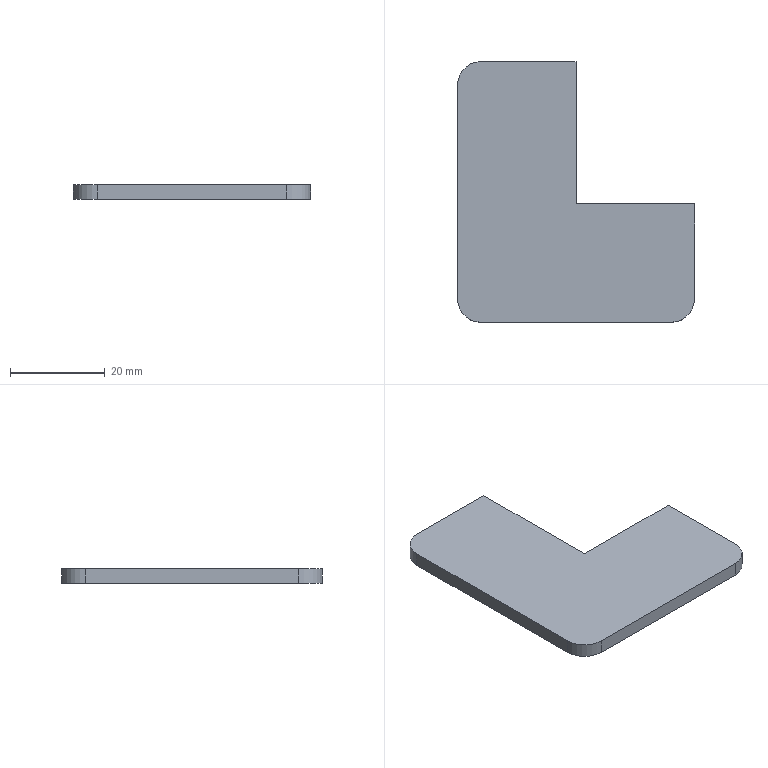Part | SolidWorks | features Extrusion 1 | 1 solid | 11 faces | box 50 x 55 x 3 mm | volume 5952 mm3 | plane 8 | cylinder 3 | commonest cylinder face diameters 10 x3
STEP:
#1=CARTESIAN_POINT('',(-360.,-23.,0.));
#2=VERTEX_POINT('',#1);
#3=CARTESIAN_POINT('',(-360.,-3.,0.));
#4=VERTEX_POINT('',#3);
#5=CARTESIAN_POINT('',(-360.,-3.,0.));
#6=DIRECTION('',(0.,1.,0.));
#7=VECTOR('',#6,1000.);
#8=LINE('',#5,#7);
#9=EDGE_CURVE('',#2,#4,#8,.T.);
#10=ORIENTED_EDGE('',*,*,#9,.T.);
#11=CARTESIAN_POINT('',(-360.,-3.,3.));
#12=VERTEX_POINT('',#11);
#13=CARTESIAN_POINT('',(-360.,-3.,3.));
#14=DIRECTION('',(0.,0.,-1.));
#15=VECTOR('',#14,1000.);
#16=LINE('',#13,#15);
#17=EDGE_CURVE('',#12,#4,#16,.T.);
#18=ORIENTED_EDGE('',*,*,#17,.F.);
#19=CARTESIAN_POINT('',(-360.,-23.,3.));
#20=VERTEX_POINT('',#19);
#21=CARTESIAN_POINT('',(-360.,-3.,3.));
#22=DIRECTION('',(0.,1.,0.));
#23=VECTOR('',#22,1000.);
#24=LINE('',#21,#23);
#25=EDGE_CURVE('',#20,#12,#24,.T.);
#26=ORIENTED_EDGE('',*,*,#25,.F.);
#27=CARTESIAN_POINT('',(-360.,-23.,3.));
#28=DIRECTION('',(0.,0.,-1.));
#29=VECTOR('',#28,1000.);
#30=LINE('',#27,#29);
#31=EDGE_CURVE('',#20,#2,#30,.T.);
#32=ORIENTED_EDGE('',*,*,#31,.T.);
#33=EDGE_LOOP('',(#10,#18,#26,#32));
#34=FACE_OUTER_BOUND('',#33,.T.);
#35=CARTESIAN_POINT('',(-360.,-3.,3.));
#36=DIRECTION('',(-1.,0.,0.));
#37=DIRECTION('',(0.,0.,1.));
#38=AXIS2_PLACEMENT_3D('',#35,#36,#37);
#39=PLANE('',#38);
#40=ADVANCED_FACE('',(#34),#39,.F.);
#41=CARTESIAN_POINT('',(-385.,-3.,0.));
#42=VERTEX_POINT('',#41);
#43=CARTESIAN_POINT('',(-360.,-3.,0.));
#44=DIRECTION('',(-1.,0.,0.));
#45=VECTOR('',#44,1000.);
#46=LINE('',#43,#45);
#47=EDGE_CURVE('',#4,#42,#46,.T.);
#48=ORIENTED_EDGE('',*,*,#47,.T.);
#49=CARTESIAN_POINT('',(-385.,-3.,3.));
#50=VERTEX_POINT('',#49);
#51=CARTESIAN_POINT('',(-385.,-3.,3.));
#52=DIRECTION('',(0.,0.,-1.));
#53=VECTOR('',#52,1000.);
#54=LINE('',#51,#53);
#55=EDGE_CURVE('',#50,#42,#54,.T.);
#56=ORIENTED_EDGE('',*,*,#55,.F.);
#57=CARTESIAN_POINT('',(-360.,-3.,3.));
#58=DIRECTION('',(-1.,0.,0.));
#59=VECTOR('',#58,1000.);
#60=LINE('',#57,#59);
#61=EDGE_CURVE('',#12,#50,#60,.T.);
#62=ORIENTED_EDGE('',*,*,#61,.F.);
#63=ORIENTED_EDGE('',*,*,#17,.T.);
#64=EDGE_LOOP('',(#48,#56,#62,#63));
#65=FACE_OUTER_BOUND('',#64,.T.);
#66=CARTESIAN_POINT('',(-360.,-3.,3.));
#67=DIRECTION('',(0.,-1.,0.));
#68=DIRECTION('',(1.,0.,0.));
#69=AXIS2_PLACEMENT_3D('',#66,#67,#68);
#70=PLANE('',#69);
#71=ADVANCED_FACE('',(#65),#70,.F.);
#72=CARTESIAN_POINT('',(-385.,27.,0.));
#73=VERTEX_POINT('',#72);
#74=CARTESIAN_POINT('',(-385.,27.,0.));
#75=DIRECTION('',(0.,1.,0.));
#76=VECTOR('',#75,1000.);
#77=LINE('',#74,#76);
#78=EDGE_CURVE('',#42,#73,#77,.T.);
#79=ORIENTED_EDGE('',*,*,#78,.T.);
#80=CARTESIAN_POINT('',(-385.,27.,3.));
#81=VERTEX_POINT('',#80);
#82=CARTESIAN_POINT('',(-385.,27.,3.));
#83=DIRECTION('',(0.,0.,-1.));
#84=VECTOR('',#83,1000.);
#85=LINE('',#82,#84);
#86=EDGE_CURVE('',#81,#73,#85,.T.);
#87=ORIENTED_EDGE('',*,*,#86,.F.);
#88=CARTESIAN_POINT('',(-385.,27.,3.));
#89=DIRECTION('',(0.,1.,0.));
#90=VECTOR('',#89,1000.);
#91=LINE('',#88,#90);
#92=EDGE_CURVE('',#50,#81,#91,.T.);
#93=ORIENTED_EDGE('',*,*,#92,.F.);
#94=ORIENTED_EDGE('',*,*,#55,.T.);
#95=EDGE_LOOP('',(#79,#87,#93,#94));
#96=FACE_OUTER_BOUND('',#95,.T.);
#97=CARTESIAN_POINT('',(-385.,27.,3.));
#98=DIRECTION('',(-1.,0.,0.));
#99=DIRECTION('',(0.,0.,1.));
#100=AXIS2_PLACEMENT_3D('',#97,#98,#99);
#101=PLANE('',#100);
#102=ADVANCED_FACE('',(#96),#101,.F.);
#103=CARTESIAN_POINT('',(-405.,27.,0.));
#104=VERTEX_POINT('',#103);
#105=CARTESIAN_POINT('',(-385.,27.,0.));
#106=DIRECTION('',(-1.,0.,0.));
#107=VECTOR('',#106,1000.);
#108=LINE('',#105,#107);
#109=EDGE_CURVE('',#73,#104,#108,.T.);
#110=ORIENTED_EDGE('',*,*,#109,.T.);
#111=CARTESIAN_POINT('',(-405.,27.,3.));
#112=VERTEX_POINT('',#111);
#113=CARTESIAN_POINT('',(-405.,27.,3.));
#114=DIRECTION('',(0.,0.,-1.));
#115=VECTOR('',#114,1000.);
#116=LINE('',#113,#115);
#117=EDGE_CURVE('',#112,#104,#116,.T.);
#118=ORIENTED_EDGE('',*,*,#117,.F.);
#119=CARTESIAN_POINT('',(-385.,27.,3.));
#120=DIRECTION('',(-1.,0.,0.));
#121=VECTOR('',#120,1000.);
#122=LINE('',#119,#121);
#123=EDGE_CURVE('',#81,#112,#122,.T.);
#124=ORIENTED_EDGE('',*,*,#123,.F.);
#125=ORIENTED_EDGE('',*,*,#86,.T.);
#126=EDGE_LOOP('',(#110,#118,#124,#125));
#127=FACE_OUTER_BOUND('',#126,.T.);
#128=CARTESIAN_POINT('',(-385.,27.,3.));
#129=DIRECTION('',(0.,-1.,0.));
#130=DIRECTION('',(1.,0.,0.));
#131=AXIS2_PLACEMENT_3D('',#128,#129,#130);
#132=PLANE('',#131);
#133=ADVANCED_FACE('',(#127),#132,.F.);
#134=CARTESIAN_POINT('',(-410.,22.,0.));
#135=VERTEX_POINT('',#134);
#136=CARTESIAN_POINT('',(-405.,22.,0.));
#137=DIRECTION('',(0.,0.,1.));
#138=DIRECTION('',(1.,0.,0.));
#139=AXIS2_PLACEMENT_3D('',#136,#137,#138);
#140=CIRCLE('',#139,5.);
#141=EDGE_CURVE('',#104,#135,#140,.T.);
#142=ORIENTED_EDGE('',*,*,#141,.T.);
#143=CARTESIAN_POINT('',(-410.,22.,3.));
#144=VERTEX_POINT('',#143);
#145=CARTESIAN_POINT('',(-410.,22.,3.));
#146=DIRECTION('',(0.,0.,-1.));
#147=VECTOR('',#146,1000.);
#148=LINE('',#145,#147);
#149=EDGE_CURVE('',#144,#135,#148,.T.);
#150=ORIENTED_EDGE('',*,*,#149,.F.);
#151=CARTESIAN_POINT('',(-405.,22.,3.));
#152=DIRECTION('',(0.,0.,1.));
#153=DIRECTION('',(1.,0.,0.));
#154=AXIS2_PLACEMENT_3D('',#151,#152,#153);
#155=CIRCLE('',#154,5.);
#156=EDGE_CURVE('',#112,#144,#155,.T.);
#157=ORIENTED_EDGE('',*,*,#156,.F.);
#158=ORIENTED_EDGE('',*,*,#117,.T.);
#159=EDGE_LOOP('',(#142,#150,#157,#158));
#160=FACE_OUTER_BOUND('',#159,.T.);
#161=CARTESIAN_POINT('',(-405.,22.,3.));
#162=DIRECTION('',(0.,0.,-1.));
#163=DIRECTION('',(-1.,0.,0.));
#164=AXIS2_PLACEMENT_3D('',#161,#162,#163);
#165=CYLINDRICAL_SURFACE('',#164,5.);
#166=ADVANCED_FACE('',(#160),#165,.T.);
#167=CARTESIAN_POINT('',(-410.,-23.,0.));
#168=VERTEX_POINT('',#167);
#169=CARTESIAN_POINT('',(-410.,-3.,0.));
#170=DIRECTION('',(0.,-1.,0.));
#171=VECTOR('',#170,1000.);
#172=LINE('',#169,#171);
#173=EDGE_CURVE('',#135,#168,#172,.T.);
#174=ORIENTED_EDGE('',*,*,#173,.T.);
#175=CARTESIAN_POINT('',(-410.,-23.,3.));
#176=VERTEX_POINT('',#175);
#177=CARTESIAN_POINT('',(-410.,-23.,3.));
#178=DIRECTION('',(0.,0.,-1.));
#179=VECTOR('',#178,1000.);
#180=LINE('',#177,#179);
#181=EDGE_CURVE('',#176,#168,#180,.T.);
#182=ORIENTED_EDGE('',*,*,#181,.F.);
#183=CARTESIAN_POINT('',(-410.,22.,3.));
#184=DIRECTION('',(0.,-1.,0.));
#185=VECTOR('',#184,1000.);
#186=LINE('',#183,#185);
#187=EDGE_CURVE('',#144,#176,#186,.T.);
#188=ORIENTED_EDGE('',*,*,#187,.F.);
#189=ORIENTED_EDGE('',*,*,#149,.T.);
#190=EDGE_LOOP('',(#174,#182,#188,#189));
#191=FACE_OUTER_BOUND('',#190,.T.);
#192=CARTESIAN_POINT('',(-410.,-3.,3.));
#193=DIRECTION('',(1.,0.,0.));
#194=DIRECTION('',(0.,0.,-1.));
#195=AXIS2_PLACEMENT_3D('',#192,#193,#194);
#196=PLANE('',#195);
#197=ADVANCED_FACE('',(#191),#196,.F.);
#198=CARTESIAN_POINT('',(-405.,-28.,0.));
#199=VERTEX_POINT('',#198);
#200=CARTESIAN_POINT('',(-405.,-23.,0.));
#201=DIRECTION('',(0.,0.,1.));
#202=DIRECTION('',(-1.,0.,0.));
#203=AXIS2_PLACEMENT_3D('',#200,#201,#202);
#204=CIRCLE('',#203,5.);
#205=EDGE_CURVE('',#168,#199,#204,.T.);
#206=ORIENTED_EDGE('',*,*,#205,.T.);
#207=CARTESIAN_POINT('',(-405.,-28.,3.));
#208=VERTEX_POINT('',#207);
#209=CARTESIAN_POINT('',(-405.,-28.,3.));
#210=DIRECTION('',(0.,0.,-1.));
#211=VECTOR('',#210,1000.);
#212=LINE('',#209,#211);
#213=EDGE_CURVE('',#208,#199,#212,.T.);
#214=ORIENTED_EDGE('',*,*,#213,.F.);
#215=CARTESIAN_POINT('',(-405.,-23.,3.));
#216=DIRECTION('',(0.,0.,1.));
#217=DIRECTION('',(-1.,0.,0.));
#218=AXIS2_PLACEMENT_3D('',#215,#216,#217);
#219=CIRCLE('',#218,5.);
#220=EDGE_CURVE('',#176,#208,#219,.T.);
#221=ORIENTED_EDGE('',*,*,#220,.F.);
#222=ORIENTED_EDGE('',*,*,#181,.T.);
#223=EDGE_LOOP('',(#206,#214,#221,#222));
#224=FACE_OUTER_BOUND('',#223,.T.);
#225=CARTESIAN_POINT('',(-405.,-23.,3.));
#226=DIRECTION('',(0.,0.,-1.));
#227=DIRECTION('',(-1.,0.,0.));
#228=AXIS2_PLACEMENT_3D('',#225,#226,#227);
#229=CYLINDRICAL_SURFACE('',#228,5.);
#230=ADVANCED_FACE('',(#224),#229,.T.);
#231=CARTESIAN_POINT('',(-365.,-28.,0.));
#232=VERTEX_POINT('',#231);
#233=CARTESIAN_POINT('',(-365.,-28.,0.));
#234=DIRECTION('',(1.,0.,0.));
#235=VECTOR('',#234,1000.);
#236=LINE('',#233,#235);
#237=EDGE_CURVE('',#199,#232,#236,.T.);
#238=ORIENTED_EDGE('',*,*,#237,.T.);
#239=CARTESIAN_POINT('',(-365.,-28.,3.));
#240=VERTEX_POINT('',#239);
#241=CARTESIAN_POINT('',(-365.,-28.,3.));
#242=DIRECTION('',(0.,0.,-1.));
#243=VECTOR('',#242,1000.);
#244=LINE('',#241,#243);
#245=EDGE_CURVE('',#240,#232,#244,.T.);
#246=ORIENTED_EDGE('',*,*,#245,.F.);
#247=CARTESIAN_POINT('',(-365.,-28.,3.));
#248=DIRECTION('',(1.,0.,0.));
#249=VECTOR('',#248,1000.);
#250=LINE('',#247,#249);
#251=EDGE_CURVE('',#208,#240,#250,.T.);
#252=ORIENTED_EDGE('',*,*,#251,.F.);
#253=ORIENTED_EDGE('',*,*,#213,.T.);
#254=EDGE_LOOP('',(#238,#246,#252,#253));
#255=FACE_OUTER_BOUND('',#254,.T.);
#256=CARTESIAN_POINT('',(-365.,-28.,3.));
#257=DIRECTION('',(0.,1.,0.));
#258=DIRECTION('',(-1.,0.,0.));
#259=AXIS2_PLACEMENT_3D('',#256,#257,#258);
#260=PLANE('',#259);
#261=ADVANCED_FACE('',(#255),#260,.F.);
#262=CARTESIAN_POINT('',(-365.,-23.,0.));
#263=DIRECTION('',(0.,0.,1.));
#264=DIRECTION('',(-1.,0.,0.));
#265=AXIS2_PLACEMENT_3D('',#262,#263,#264);
#266=CIRCLE('',#265,5.);
#267=EDGE_CURVE('',#232,#2,#266,.T.);
#268=ORIENTED_EDGE('',*,*,#267,.T.);
#269=ORIENTED_EDGE('',*,*,#31,.F.);
#270=CARTESIAN_POINT('',(-365.,-23.,3.));
#271=DIRECTION('',(0.,0.,1.));
#272=DIRECTION('',(-1.,0.,0.));
#273=AXIS2_PLACEMENT_3D('',#270,#271,#272);
#274=CIRCLE('',#273,5.);
#275=EDGE_CURVE('',#240,#20,#274,.T.);
#276=ORIENTED_EDGE('',*,*,#275,.F.);
#277=ORIENTED_EDGE('',*,*,#245,.T.);
#278=EDGE_LOOP('',(#268,#269,#276,#277));
#279=FACE_OUTER_BOUND('',#278,.T.);
#280=CARTESIAN_POINT('',(-365.,-23.,3.));
#281=DIRECTION('',(0.,0.,-1.));
#282=DIRECTION('',(-1.,0.,0.));
#283=AXIS2_PLACEMENT_3D('',#280,#281,#282);
#284=CYLINDRICAL_SURFACE('',#283,5.);
#285=ADVANCED_FACE('',(#279),#284,.T.);
#286=ORIENTED_EDGE('',*,*,#25,.T.);
#287=ORIENTED_EDGE('',*,*,#61,.T.);
#288=ORIENTED_EDGE('',*,*,#92,.T.);
#289=ORIENTED_EDGE('',*,*,#123,.T.);
#290=ORIENTED_EDGE('',*,*,#156,.T.);
#291=ORIENTED_EDGE('',*,*,#187,.T.);
#292=ORIENTED_EDGE('',*,*,#220,.T.);
#293=ORIENTED_EDGE('',*,*,#251,.T.);
#294=ORIENTED_EDGE('',*,*,#275,.T.);
#295=EDGE_LOOP('',(#286,#287,#288,#289,#290,#291,#292,#293,#294));
#296=FACE_OUTER_BOUND('',#295,.T.);
#297=CARTESIAN_POINT('',(-365.,-23.,3.));
#298=DIRECTION('',(0.,0.,-1.));
#299=DIRECTION('',(-1.,0.,0.));
#300=AXIS2_PLACEMENT_3D('',#297,#298,#299);
#301=PLANE('',#300);
#302=ADVANCED_FACE('',(#296),#301,.F.);
#303=ORIENTED_EDGE('',*,*,#9,.F.);
#304=ORIENTED_EDGE('',*,*,#267,.F.);
#305=ORIENTED_EDGE('',*,*,#237,.F.);
#306=ORIENTED_EDGE('',*,*,#205,.F.);
#307=ORIENTED_EDGE('',*,*,#173,.F.);
#308=ORIENTED_EDGE('',*,*,#141,.F.);
#309=ORIENTED_EDGE('',*,*,#109,.F.);
#310=ORIENTED_EDGE('',*,*,#78,.F.);
#311=ORIENTED_EDGE('',*,*,#47,.F.);
#312=EDGE_LOOP('',(#303,#304,#305,#306,#307,#308,#309,#310,#311));
#313=FACE_OUTER_BOUND('',#312,.T.);
#314=CARTESIAN_POINT('',(-365.,-23.,0.));
#315=DIRECTION('',(0.,0.,-1.));
#316=DIRECTION('',(-1.,0.,0.));
#317=AXIS2_PLACEMENT_3D('',#314,#315,#316);
#318=PLANE('',#317);
#319=ADVANCED_FACE('',(#313),#318,.T.);
#320=CLOSED_SHELL('',(#40,#71,#102,#133,#166,#197,#230,#261,#285,#302,#319));
#321=MANIFOLD_SOLID_BREP('',#320);
#322=CARTESIAN_POINT('',(0.,0.,0.));
#323=DIRECTION('',(0.,0.,1.));
#324=DIRECTION('',(1.,0.,0.));
#325=AXIS2_PLACEMENT_3D('',#322,#323,#324);
#326=(LENGTH_UNIT()NAMED_UNIT(*)SI_UNIT(.MILLI.,.METRE.));
#327=UNCERTAINTY_MEASURE_WITH_UNIT(LENGTH_MEASURE(0.00001),#326,'','');
#328=(NAMED_UNIT(*)PLANE_ANGLE_UNIT()SI_UNIT($,.RADIAN.));
#329=(NAMED_UNIT(*)SI_UNIT($,.STERADIAN.)SOLID_ANGLE_UNIT());
#330=(GEOMETRIC_REPRESENTATION_CONTEXT(3)GLOBAL_UNCERTAINTY_ASSIGNED_CONTEXT((#327))GLOBAL_UNIT_ASSIGNED_CONTEXT((#326,#328,#329))REPRESENTATION_CONTEXT('',''));
#331=ADVANCED_BREP_SHAPE_REPRESENTATION('',(#321,#325),#330);